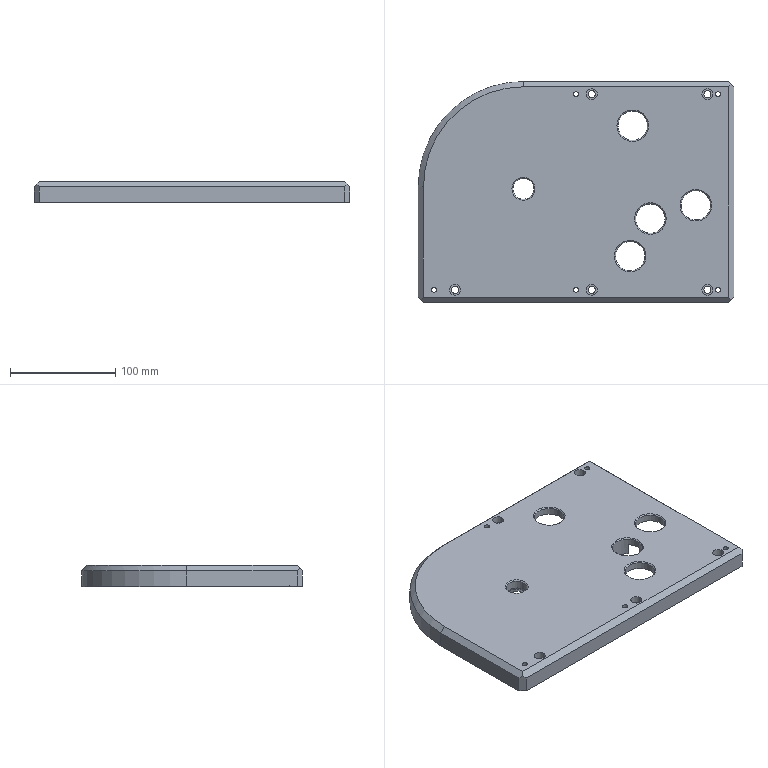Part | NX | features BREP 1 | 1 solid | 88 faces | box 300 x 210 x 20 mm | volume 677467 mm3 | cylinder 43 | plane 31 | cone 8 | torus 6 | commonest cylinder face diameters 67 x7 5 x5 6.6 x5 10.5 x5 3 x4 28 x4